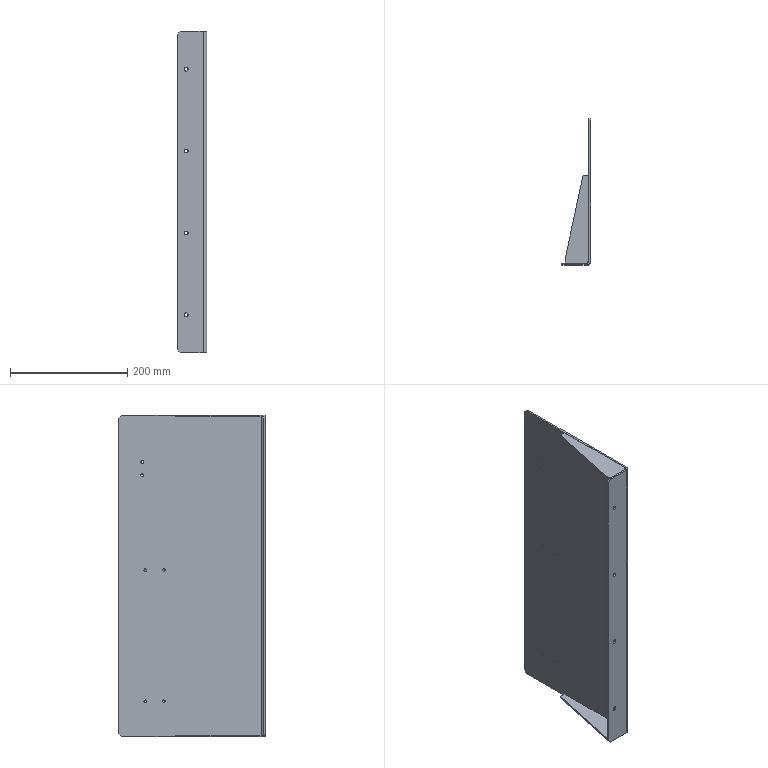Part | SolidWorks | features BaseBody 3 | 3 solids | 50 faces | box 50 x 250 x 550 mm | volume 509344 mm3 | plane 28 | cylinder 22 | commonest cylinder face diameters 4.2 x8 6.6 x8 5 x4 6 x1 12 x1
STEP:
#1=CARTESIAN_POINT('',(-3.,8.,272.));
#2=VERTEX_POINT('',#1);
#3=CARTESIAN_POINT('',(-8.,3.,272.));
#4=VERTEX_POINT('',#3);
#5=CARTESIAN_POINT('',(-5.5,5.5,272.));
#6=DIRECTION('',(-0.7071,-0.7071,0.));
#7=VECTOR('',#6,1000.);
#8=LINE('',#5,#7);
#9=EDGE_CURVE('',#2,#4,#8,.T.);
#10=ORIENTED_EDGE('',*,*,#9,.F.);
#11=CARTESIAN_POINT('',(-3.,8.,275.));
#12=VERTEX_POINT('',#11);
#13=CARTESIAN_POINT('',(-3.,8.,272.));
#14=DIRECTION('',(0.,0.,-1.));
#15=VECTOR('',#14,1000.);
#16=LINE('',#13,#15);
#17=EDGE_CURVE('',#12,#2,#16,.T.);
#18=ORIENTED_EDGE('',*,*,#17,.F.);
#19=CARTESIAN_POINT('',(-8.,3.,275.));
#20=VERTEX_POINT('',#19);
#21=CARTESIAN_POINT('',(-8.,3.,275.));
#22=DIRECTION('',(0.7071,0.7071,0.));
#23=VECTOR('',#22,1000.);
#24=LINE('',#21,#23);
#25=EDGE_CURVE('',#20,#12,#24,.T.);
#26=ORIENTED_EDGE('',*,*,#25,.F.);
#27=CARTESIAN_POINT('',(-8.,3.,272.));
#28=DIRECTION('',(0.,0.,1.));
#29=VECTOR('',#28,1000.);
#30=LINE('',#27,#29);
#31=EDGE_CURVE('',#4,#20,#30,.T.);
#32=ORIENTED_EDGE('',*,*,#31,.F.);
#33=EDGE_LOOP('',(#10,#18,#26,#32));
#34=FACE_OUTER_BOUND('',#33,.T.);
#35=CARTESIAN_POINT('',(-8.,3.,272.));
#36=DIRECTION('',(-0.7071,0.7071,0.));
#37=DIRECTION('',(0.,0.,1.));
#38=AXIS2_PLACEMENT_3D('',#35,#36,#37);
#39=PLANE('',#38);
#40=ADVANCED_FACE('',(#34),#39,.F.);
#41=CARTESIAN_POINT('',(-43.,3.,275.));
#42=VERTEX_POINT('',#41);
#43=CARTESIAN_POINT('',(-3.,3.,275.));
#44=DIRECTION('',(-1.,0.,0.));
#45=VECTOR('',#44,1000.);
#46=LINE('',#43,#45);
#47=EDGE_CURVE('',#20,#42,#46,.T.);
#48=ORIENTED_EDGE('',*,*,#47,.F.);
#49=ORIENTED_EDGE('',*,*,#25,.T.);
#50=CARTESIAN_POINT('',(-3.,153.,275.));
#51=VERTEX_POINT('',#50);
#52=CARTESIAN_POINT('',(-3.,3.,275.));
#53=DIRECTION('',(0.,-1.,0.));
#54=VECTOR('',#53,1000.);
#55=LINE('',#52,#54);
#56=EDGE_CURVE('',#51,#12,#55,.T.);
#57=ORIENTED_EDGE('',*,*,#56,.F.);
#58=CARTESIAN_POINT('',(-13.,153.,275.));
#59=VERTEX_POINT('',#58);
#60=CARTESIAN_POINT('',(-3.,153.,275.));
#61=DIRECTION('',(1.,0.,0.));
#62=VECTOR('',#61,1000.);
#63=LINE('',#60,#62);
#64=EDGE_CURVE('',#59,#51,#63,.T.);
#65=ORIENTED_EDGE('',*,*,#64,.F.);
#66=CARTESIAN_POINT('',(-43.,13.,275.));
#67=VERTEX_POINT('',#66);
#68=CARTESIAN_POINT('',(-13.,153.,275.));
#69=DIRECTION('',(0.2095,0.9778,0.));
#70=VECTOR('',#69,1000.);
#71=LINE('',#68,#70);
#72=EDGE_CURVE('',#67,#59,#71,.T.);
#73=ORIENTED_EDGE('',*,*,#72,.F.);
#74=CARTESIAN_POINT('',(-43.,3.,275.));
#75=DIRECTION('',(0.,1.,0.));
#76=VECTOR('',#75,1000.);
#77=LINE('',#74,#76);
#78=EDGE_CURVE('',#42,#67,#77,.T.);
#79=ORIENTED_EDGE('',*,*,#78,.F.);
#80=EDGE_LOOP('',(#48,#49,#57,#65,#73,#79));
#81=FACE_OUTER_BOUND('',#80,.T.);
#82=CARTESIAN_POINT('',(0.,0.,275.));
#83=DIRECTION('',(0.,0.,-1.));
#84=DIRECTION('',(-1.,0.,0.));
#85=AXIS2_PLACEMENT_3D('',#82,#83,#84);
#86=PLANE('',#85);
#87=ADVANCED_FACE('',(#81),#86,.F.);
#88=CARTESIAN_POINT('',(-3.,153.,272.));
#89=VERTEX_POINT('',#88);
#90=CARTESIAN_POINT('',(-3.,3.,272.));
#91=DIRECTION('',(0.,-1.,0.));
#92=VECTOR('',#91,1000.);
#93=LINE('',#90,#92);
#94=EDGE_CURVE('',#89,#2,#93,.T.);
#95=ORIENTED_EDGE('',*,*,#94,.T.);
#96=ORIENTED_EDGE('',*,*,#9,.T.);
#97=CARTESIAN_POINT('',(-43.,3.,272.));
#98=VERTEX_POINT('',#97);
#99=CARTESIAN_POINT('',(-3.,3.,272.));
#100=DIRECTION('',(-1.,0.,0.));
#101=VECTOR('',#100,1000.);
#102=LINE('',#99,#101);
#103=EDGE_CURVE('',#4,#98,#102,.T.);
#104=ORIENTED_EDGE('',*,*,#103,.T.);
#105=CARTESIAN_POINT('',(-43.,13.,272.));
#106=VERTEX_POINT('',#105);
#107=CARTESIAN_POINT('',(-43.,3.,272.));
#108=DIRECTION('',(0.,1.,0.));
#109=VECTOR('',#108,1000.);
#110=LINE('',#107,#109);
#111=EDGE_CURVE('',#98,#106,#110,.T.);
#112=ORIENTED_EDGE('',*,*,#111,.T.);
#113=CARTESIAN_POINT('',(-13.,153.,272.));
#114=VERTEX_POINT('',#113);
#115=CARTESIAN_POINT('',(-13.,153.,272.));
#116=DIRECTION('',(0.2095,0.9778,0.));
#117=VECTOR('',#116,1000.);
#118=LINE('',#115,#117);
#119=EDGE_CURVE('',#106,#114,#118,.T.);
#120=ORIENTED_EDGE('',*,*,#119,.T.);
#121=CARTESIAN_POINT('',(-3.,153.,272.));
#122=DIRECTION('',(1.,0.,0.));
#123=VECTOR('',#122,1000.);
#124=LINE('',#121,#123);
#125=EDGE_CURVE('',#114,#89,#124,.T.);
#126=ORIENTED_EDGE('',*,*,#125,.T.);
#127=EDGE_LOOP('',(#95,#96,#104,#112,#120,#126));
#128=FACE_OUTER_BOUND('',#127,.T.);
#129=CARTESIAN_POINT('',(0.,0.,272.));
#130=DIRECTION('',(0.,0.,-1.));
#131=DIRECTION('',(-1.,0.,0.));
#132=AXIS2_PLACEMENT_3D('',#129,#130,#131);
#133=PLANE('',#132);
#134=ADVANCED_FACE('',(#128),#133,.T.);
#135=ORIENTED_EDGE('',*,*,#72,.T.);
#136=CARTESIAN_POINT('',(-13.,153.,272.));
#137=DIRECTION('',(0.,0.,1.));
#138=VECTOR('',#137,1000.);
#139=LINE('',#136,#138);
#140=EDGE_CURVE('',#114,#59,#139,.T.);
#141=ORIENTED_EDGE('',*,*,#140,.F.);
#142=ORIENTED_EDGE('',*,*,#119,.F.);
#143=CARTESIAN_POINT('',(-43.,13.,272.));
#144=DIRECTION('',(0.,0.,1.));
#145=VECTOR('',#144,1000.);
#146=LINE('',#143,#145);
#147=EDGE_CURVE('',#106,#67,#146,.T.);
#148=ORIENTED_EDGE('',*,*,#147,.T.);
#149=EDGE_LOOP('',(#135,#141,#142,#148));
#150=FACE_OUTER_BOUND('',#149,.T.);
#151=CARTESIAN_POINT('',(-13.,153.,272.));
#152=DIRECTION('',(0.9778,-0.2095,0.));
#153=DIRECTION('',(0.,0.,-1.));
#154=AXIS2_PLACEMENT_3D('',#151,#152,#153);
#155=PLANE('',#154);
#156=ADVANCED_FACE('',(#150),#155,.F.);
#157=ORIENTED_EDGE('',*,*,#78,.T.);
#158=ORIENTED_EDGE('',*,*,#147,.F.);
#159=ORIENTED_EDGE('',*,*,#111,.F.);
#160=CARTESIAN_POINT('',(-43.,3.,272.));
#161=DIRECTION('',(0.,0.,1.));
#162=VECTOR('',#161,1000.);
#163=LINE('',#160,#162);
#164=EDGE_CURVE('',#98,#42,#163,.T.);
#165=ORIENTED_EDGE('',*,*,#164,.T.);
#166=EDGE_LOOP('',(#157,#158,#159,#165));
#167=FACE_OUTER_BOUND('',#166,.T.);
#168=CARTESIAN_POINT('',(-43.,3.,272.));
#169=DIRECTION('',(1.,0.,0.));
#170=DIRECTION('',(0.,1.,0.));
#171=AXIS2_PLACEMENT_3D('',#168,#169,#170);
#172=PLANE('',#171);
#173=ADVANCED_FACE('',(#167),#172,.F.);
#174=ORIENTED_EDGE('',*,*,#103,.F.);
#175=ORIENTED_EDGE('',*,*,#31,.T.);
#176=ORIENTED_EDGE('',*,*,#47,.T.);
#177=ORIENTED_EDGE('',*,*,#164,.F.);
#178=EDGE_LOOP('',(#174,#175,#176,#177));
#179=FACE_OUTER_BOUND('',#178,.T.);
#180=CARTESIAN_POINT('',(-3.,3.,272.));
#181=DIRECTION('',(0.,1.,0.));
#182=DIRECTION('',(1.,0.,0.));
#183=AXIS2_PLACEMENT_3D('',#180,#181,#182);
#184=PLANE('',#183);
#185=ADVANCED_FACE('',(#179),#184,.F.);
#186=ORIENTED_EDGE('',*,*,#56,.T.);
#187=ORIENTED_EDGE('',*,*,#17,.T.);
#188=ORIENTED_EDGE('',*,*,#94,.F.);
#189=CARTESIAN_POINT('',(-3.,153.,272.));
#190=DIRECTION('',(0.,0.,1.));
#191=VECTOR('',#190,1000.);
#192=LINE('',#189,#191);
#193=EDGE_CURVE('',#89,#51,#192,.T.);
#194=ORIENTED_EDGE('',*,*,#193,.T.);
#195=EDGE_LOOP('',(#186,#187,#188,#194));
#196=FACE_OUTER_BOUND('',#195,.T.);
#197=CARTESIAN_POINT('',(-3.,3.,272.));
#198=DIRECTION('',(-1.,0.,0.));
#199=DIRECTION('',(0.,1.,0.));
#200=AXIS2_PLACEMENT_3D('',#197,#198,#199);
#201=PLANE('',#200);
#202=ADVANCED_FACE('',(#196),#201,.F.);
#203=ORIENTED_EDGE('',*,*,#64,.T.);
#204=ORIENTED_EDGE('',*,*,#193,.F.);
#205=ORIENTED_EDGE('',*,*,#125,.F.);
#206=ORIENTED_EDGE('',*,*,#140,.T.);
#207=EDGE_LOOP('',(#203,#204,#205,#206));
#208=FACE_OUTER_BOUND('',#207,.T.);
#209=CARTESIAN_POINT('',(-3.,153.,272.));
#210=DIRECTION('',(0.,-1.,0.));
#211=DIRECTION('',(-1.,0.,0.));
#212=AXIS2_PLACEMENT_3D('',#209,#210,#211);
#213=PLANE('',#212);
#214=ADVANCED_FACE('',(#208),#213,.F.);
#215=CLOSED_SHELL('',(#40,#87,#134,#156,#173,#185,#202,#214));
#216=MANIFOLD_SOLID_BREP('',#215);
#217=CARTESIAN_POINT('',(-8.,3.,-272.));
#218=VERTEX_POINT('',#217);
#219=CARTESIAN_POINT('',(-3.,8.,-272.));
#220=VERTEX_POINT('',#219);
#221=CARTESIAN_POINT('',(-3.,8.,-272.));
#222=DIRECTION('',(0.7071,0.7071,0.));
#223=VECTOR('',#222,1000.);
#224=LINE('',#221,#223);
#225=EDGE_CURVE('',#218,#220,#224,.T.);
#226=ORIENTED_EDGE('',*,*,#225,.F.);
#227=CARTESIAN_POINT('',(-8.,3.,-275.));
#228=VERTEX_POINT('',#227);
#229=CARTESIAN_POINT('',(-8.,3.,-272.));
#230=DIRECTION('',(0.,0.,1.));
#231=VECTOR('',#230,1000.);
#232=LINE('',#229,#231);
#233=EDGE_CURVE('',#228,#218,#232,.T.);
#234=ORIENTED_EDGE('',*,*,#233,.F.);
#235=CARTESIAN_POINT('',(-3.,8.,-275.));
#236=VERTEX_POINT('',#235);
#237=CARTESIAN_POINT('',(-5.5,5.5,-275.));
#238=DIRECTION('',(-0.7071,-0.7071,0.));
#239=VECTOR('',#238,1000.);
#240=LINE('',#237,#239);
#241=EDGE_CURVE('',#236,#228,#240,.T.);
#242=ORIENTED_EDGE('',*,*,#241,.F.);
#243=CARTESIAN_POINT('',(-3.,8.,-272.));
#244=DIRECTION('',(0.,0.,-1.));
#245=VECTOR('',#244,1000.);
#246=LINE('',#243,#245);
#247=EDGE_CURVE('',#220,#236,#246,.T.);
#248=ORIENTED_EDGE('',*,*,#247,.F.);
#249=EDGE_LOOP('',(#226,#234,#242,#248));
#250=FACE_OUTER_BOUND('',#249,.T.);
#251=CARTESIAN_POINT('',(-3.,8.,-272.));
#252=DIRECTION('',(-0.7071,0.7071,0.));
#253=DIRECTION('',(0.,0.,1.));
#254=AXIS2_PLACEMENT_3D('',#251,#252,#253);
#255=PLANE('',#254);
#256=ADVANCED_FACE('',(#250),#255,.F.);
#257=CARTESIAN_POINT('',(-3.,153.,-275.));
#258=VERTEX_POINT('',#257);
#259=CARTESIAN_POINT('',(-3.,3.,-275.));
#260=DIRECTION('',(0.,1.,0.));
#261=VECTOR('',#260,1000.);
#262=LINE('',#259,#261);
#263=EDGE_CURVE('',#236,#258,#262,.T.);
#264=ORIENTED_EDGE('',*,*,#263,.F.);
#265=ORIENTED_EDGE('',*,*,#241,.T.);
#266=CARTESIAN_POINT('',(-43.,3.,-275.));
#267=VERTEX_POINT('',#266);
#268=CARTESIAN_POINT('',(-3.,3.,-275.));
#269=DIRECTION('',(1.,0.,0.));
#270=VECTOR('',#269,1000.);
#271=LINE('',#268,#270);
#272=EDGE_CURVE('',#267,#228,#271,.T.);
#273=ORIENTED_EDGE('',*,*,#272,.F.);
#274=CARTESIAN_POINT('',(-43.,13.,-275.));
#275=VERTEX_POINT('',#274);
#276=CARTESIAN_POINT('',(-43.,3.,-275.));
#277=DIRECTION('',(0.,-1.,0.));
#278=VECTOR('',#277,1000.);
#279=LINE('',#276,#278);
#280=EDGE_CURVE('',#275,#267,#279,.T.);
#281=ORIENTED_EDGE('',*,*,#280,.F.);
#282=CARTESIAN_POINT('',(-13.,153.,-275.));
#283=VERTEX_POINT('',#282);
#284=CARTESIAN_POINT('',(-13.,153.,-275.));
#285=DIRECTION('',(-0.2095,-0.9778,0.));
#286=VECTOR('',#285,1000.);
#287=LINE('',#284,#286);
#288=EDGE_CURVE('',#283,#275,#287,.T.);
#289=ORIENTED_EDGE('',*,*,#288,.F.);
#290=CARTESIAN_POINT('',(-3.,153.,-275.));
#291=DIRECTION('',(-1.,0.,0.));
#292=VECTOR('',#291,1000.);
#293=LINE('',#290,#292);
#294=EDGE_CURVE('',#258,#283,#293,.T.);
#295=ORIENTED_EDGE('',*,*,#294,.F.);
#296=EDGE_LOOP('',(#264,#265,#273,#281,#289,#295));
#297=FACE_OUTER_BOUND('',#296,.T.);
#298=CARTESIAN_POINT('',(0.,0.,-275.));
#299=DIRECTION('',(0.,0.,-1.));
#300=DIRECTION('',(-1.,0.,0.));
#301=AXIS2_PLACEMENT_3D('',#298,#299,#300);
#302=PLANE('',#301);
#303=ADVANCED_FACE('',(#297),#302,.T.);
#304=CARTESIAN_POINT('',(-43.,3.,-272.));
#305=VERTEX_POINT('',#304);
#306=CARTESIAN_POINT('',(-3.,3.,-272.));
#307=DIRECTION('',(1.,0.,0.));
#308=VECTOR('',#307,1000.);
#309=LINE('',#306,#308);
#310=EDGE_CURVE('',#305,#218,#309,.T.);
#311=ORIENTED_EDGE('',*,*,#310,.T.);
#312=ORIENTED_EDGE('',*,*,#225,.T.);
#313=CARTESIAN_POINT('',(-3.,153.,-272.));
#314=VERTEX_POINT('',#313);
#315=CARTESIAN_POINT('',(-3.,3.,-272.));
#316=DIRECTION('',(0.,1.,0.));
#317=VECTOR('',#316,1000.);
#318=LINE('',#315,#317);
#319=EDGE_CURVE('',#220,#314,#318,.T.);
#320=ORIENTED_EDGE('',*,*,#319,.T.);
#321=CARTESIAN_POINT('',(-13.,153.,-272.));
#322=VERTEX_POINT('',#321);
#323=CARTESIAN_POINT('',(-3.,153.,-272.));
#324=DIRECTION('',(-1.,0.,0.));
#325=VECTOR('',#324,1000.);
#326=LINE('',#323,#325);
#327=EDGE_CURVE('',#314,#322,#326,.T.);
#328=ORIENTED_EDGE('',*,*,#327,.T.);
#329=CARTESIAN_POINT('',(-43.,13.,-272.));
#330=VERTEX_POINT('',#329);
#331=CARTESIAN_POINT('',(-13.,153.,-272.));
#332=DIRECTION('',(-0.2095,-0.9778,0.));
#333=VECTOR('',#332,1000.);
#334=LINE('',#331,#333);
#335=EDGE_CURVE('',#322,#330,#334,.T.);
#336=ORIENTED_EDGE('',*,*,#335,.T.);
#337=CARTESIAN_POINT('',(-43.,3.,-272.));
#338=DIRECTION('',(0.,-1.,0.));
#339=VECTOR('',#338,1000.);
#340=LINE('',#337,#339);
#341=EDGE_CURVE('',#330,#305,#340,.T.);
#342=ORIENTED_EDGE('',*,*,#341,.T.);
#343=EDGE_LOOP('',(#311,#312,#320,#328,#336,#342));
#344=FACE_OUTER_BOUND('',#343,.T.);
#345=CARTESIAN_POINT('',(0.,0.,-272.));
#346=DIRECTION('',(0.,0.,-1.));
#347=DIRECTION('',(-1.,0.,0.));
#348=AXIS2_PLACEMENT_3D('',#345,#346,#347);
#349=PLANE('',#348);
#350=ADVANCED_FACE('',(#344),#349,.F.);
#351=ORIENTED_EDGE('',*,*,#319,.F.);
#352=ORIENTED_EDGE('',*,*,#247,.T.);
#353=ORIENTED_EDGE('',*,*,#263,.T.);
#354=CARTESIAN_POINT('',(-3.,153.,-272.));
#355=DIRECTION('',(0.,0.,-1.));
#356=VECTOR('',#355,1000.);
#357=LINE('',#354,#356);
#358=EDGE_CURVE('',#314,#258,#357,.T.);
#359=ORIENTED_EDGE('',*,*,#358,.F.);
#360=EDGE_LOOP('',(#351,#352,#353,#359));
#361=FACE_OUTER_BOUND('',#360,.T.);
#362=CARTESIAN_POINT('',(-3.,3.,-272.));
#363=DIRECTION('',(-1.,0.,0.));
#364=DIRECTION('',(0.,1.,0.));
#365=AXIS2_PLACEMENT_3D('',#362,#363,#364);
#366=PLANE('',#365);
#367=ADVANCED_FACE('',(#361),#366,.F.);
#368=ORIENTED_EDGE('',*,*,#272,.T.);
#369=ORIENTED_EDGE('',*,*,#233,.T.);
#370=ORIENTED_EDGE('',*,*,#310,.F.);
#371=CARTESIAN_POINT('',(-43.,3.,-272.));
#372=DIRECTION('',(0.,0.,-1.));
#373=VECTOR('',#372,1000.);
#374=LINE('',#371,#373);
#375=EDGE_CURVE('',#305,#267,#374,.T.);
#376=ORIENTED_EDGE('',*,*,#375,.T.);
#377=EDGE_LOOP('',(#368,#369,#370,#376));
#378=FACE_OUTER_BOUND('',#377,.T.);
#379=CARTESIAN_POINT('',(-3.,3.,-272.));
#380=DIRECTION('',(0.,1.,0.));
#381=DIRECTION('',(0.,0.,-1.));
#382=AXIS2_PLACEMENT_3D('',#379,#380,#381);
#383=PLANE('',#382);
#384=ADVANCED_FACE('',(#378),#383,.F.);
#385=ORIENTED_EDGE('',*,*,#280,.T.);
#386=ORIENTED_EDGE('',*,*,#375,.F.);
#387=ORIENTED_EDGE('',*,*,#341,.F.);
#388=CARTESIAN_POINT('',(-43.,13.,-272.));
#389=DIRECTION('',(0.,0.,-1.));
#390=VECTOR('',#389,1000.);
#391=LINE('',#388,#390);
#392=EDGE_CURVE('',#330,#275,#391,.T.);
#393=ORIENTED_EDGE('',*,*,#392,.T.);
#394=EDGE_LOOP('',(#385,#386,#387,#393));
#395=FACE_OUTER_BOUND('',#394,.T.);
#396=CARTESIAN_POINT('',(-43.,3.,-272.));
#397=DIRECTION('',(1.,0.,0.));
#398=DIRECTION('',(0.,-1.,0.));
#399=AXIS2_PLACEMENT_3D('',#396,#397,#398);
#400=PLANE('',#399);
#401=ADVANCED_FACE('',(#395),#400,.F.);
#402=ORIENTED_EDGE('',*,*,#288,.T.);
#403=ORIENTED_EDGE('',*,*,#392,.F.);
#404=ORIENTED_EDGE('',*,*,#335,.F.);
#405=CARTESIAN_POINT('',(-13.,153.,-272.));
#406=DIRECTION('',(0.,0.,-1.));
#407=VECTOR('',#406,1000.);
#408=LINE('',#405,#407);
#409=EDGE_CURVE('',#322,#283,#408,.T.);
#410=ORIENTED_EDGE('',*,*,#409,.T.);
#411=EDGE_LOOP('',(#402,#403,#404,#410));
#412=FACE_OUTER_BOUND('',#411,.T.);
#413=CARTESIAN_POINT('',(-13.,153.,-272.));
#414=DIRECTION('',(0.9778,-0.2095,0.));
#415=DIRECTION('',(0.,0.,-1.));
#416=AXIS2_PLACEMENT_3D('',#413,#414,#415);
#417=PLANE('',#416);
#418=ADVANCED_FACE('',(#412),#417,.F.);
#419=ORIENTED_EDGE('',*,*,#294,.T.);
#420=ORIENTED_EDGE('',*,*,#409,.F.);
#421=ORIENTED_EDGE('',*,*,#327,.F.);
#422=ORIENTED_EDGE('',*,*,#358,.T.);
#423=EDGE_LOOP('',(#419,#420,#421,#422));
#424=FACE_OUTER_BOUND('',#423,.T.);
#425=CARTESIAN_POINT('',(-3.,153.,-272.));
#426=DIRECTION('',(0.,-1.,0.));
#427=DIRECTION('',(0.,0.,-1.));
#428=AXIS2_PLACEMENT_3D('',#425,#426,#427);
#429=PLANE('',#428);
#430=ADVANCED_FACE('',(#424),#429,.F.);
#431=CLOSED_SHELL('',(#256,#303,#350,#367,#384,#401,#418,#430));
#432=MANIFOLD_SOLID_BREP('',#431);
#433=CARTESIAN_POINT('',(-3.,210.,197.5));
#434=VERTEX_POINT('',#433);
#435=CARTESIAN_POINT('',(-3.,210.,192.5));
#436=VERTEX_POINT('',#435);
#437=CARTESIAN_POINT('',(-3.,210.,195.));
#438=DIRECTION('',(1.,0.,0.));
#439=DIRECTION('',(0.,1.,0.));
#440=AXIS2_PLACEMENT_3D('',#437,#438,#439);
#441=CIRCLE('',#440,2.5);
#442=EDGE_CURVE('',#434,#436,#441,.T.);
#443=ORIENTED_EDGE('',*,*,#442,.F.);
#444=CARTESIAN_POINT('',(0.,210.,197.5));
#445=VERTEX_POINT('',#444);
#446=CARTESIAN_POINT('',(0.,210.,197.5));
#447=DIRECTION('',(1.,0.,0.));
#448=VECTOR('',#447,1000.);
#449=LINE('',#446,#448);
#450=EDGE_CURVE('',#434,#445,#449,.T.);
#451=ORIENTED_EDGE('',*,*,#450,.T.);
#452=CARTESIAN_POINT('',(0.,210.,192.5));
#453=VERTEX_POINT('',#452);
#454=CARTESIAN_POINT('',(0.,210.,195.));
#455=DIRECTION('',(1.,0.,0.));
#456=DIRECTION('',(0.,0.,-1.));
#457=AXIS2_PLACEMENT_3D('',#454,#455,#456);
#458=CIRCLE('',#457,2.5);
#459=EDGE_CURVE('',#445,#453,#458,.T.);
#460=ORIENTED_EDGE('',*,*,#459,.T.);
#461=CARTESIAN_POINT('',(0.,210.,192.5));
#462=DIRECTION('',(1.,0.,0.));
#463=VECTOR('',#462,1000.);
#464=LINE('',#461,#463);
#465=EDGE_CURVE('',#436,#453,#464,.T.);
#466=ORIENTED_EDGE('',*,*,#465,.F.);
#467=EDGE_LOOP('',(#443,#451,#460,#466));
#468=FACE_OUTER_BOUND('',#467,.T.);
#469=CARTESIAN_POINT('',(0.,210.,195.));
#470=DIRECTION('',(1.,0.,0.));
#471=DIRECTION('',(0.,0.,-1.));
#472=AXIS2_PLACEMENT_3D('',#469,#470,#471);
#473=CYLINDRICAL_SURFACE('',#472,2.5);
#474=ADVANCED_FACE('',(#468),#473,.F.);
#475=CARTESIAN_POINT('',(-3.,210.,174.5));
#476=VERTEX_POINT('',#475);
#477=CARTESIAN_POINT('',(-3.,210.,169.5));
#478=VERTEX_POINT('',#477);
#479=CARTESIAN_POINT('',(-3.,210.,172.));
#480=DIRECTION('',(1.,0.,0.));
#481=DIRECTION('',(0.,1.,0.));
#482=AXIS2_PLACEMENT_3D('',#479,#480,#481);
#483=CIRCLE('',#482,2.5);
#484=EDGE_CURVE('',#476,#478,#483,.T.);
#485=ORIENTED_EDGE('',*,*,#484,.F.);
#486=CARTESIAN_POINT('',(0.,210.,174.5));
#487=VERTEX_POINT('',#486);
#488=CARTESIAN_POINT('',(0.,210.,174.5));
#489=DIRECTION('',(1.,0.,0.));
#490=VECTOR('',#489,1000.);
#491=LINE('',#488,#490);
#492=EDGE_CURVE('',#476,#487,#491,.T.);
#493=ORIENTED_EDGE('',*,*,#492,.T.);
#494=CARTESIAN_POINT('',(0.,210.,169.5));
#495=VERTEX_POINT('',#494);
#496=CARTESIAN_POINT('',(0.,210.,172.));
#497=DIRECTION('',(1.,0.,0.));
#498=DIRECTION('',(0.,0.,-1.));
#499=AXIS2_PLACEMENT_3D('',#496,#497,#498);
#500=CIRCLE('',#499,2.5);
#501=EDGE_CURVE('',#487,#495,#500,.T.);
#502=ORIENTED_EDGE('',*,*,#501,.T.);
#503=CARTESIAN_POINT('',(0.,210.,169.5));
#504=DIRECTION('',(1.,0.,0.));
#505=VECTOR('',#504,1000.);
#506=LINE('',#503,#505);
#507=EDGE_CURVE('',#478,#495,#506,.T.);
#508=ORIENTED_EDGE('',*,*,#507,.F.);
#509=EDGE_LOOP('',(#485,#493,#502,#508));
#510=FACE_OUTER_BOUND('',#509,.T.);
#511=CARTESIAN_POINT('',(0.,210.,172.));
#512=DIRECTION('',(1.,0.,0.));
#513=DIRECTION('',(0.,0.,-1.));
#514=AXIS2_PLACEMENT_3D('',#511,#512,#513);
#515=CYLINDRICAL_SURFACE('',#514,2.5);
#516=ADVANCED_FACE('',(#510),#515,.F.);
#517=CARTESIAN_POINT('',(-35.,0.,213.3));
#518=VERTEX_POINT('',#517);
#519=CARTESIAN_POINT('',(-35.,0.,206.7));
#520=VERTEX_POINT('',#519);
#521=CARTESIAN_POINT('',(-35.,0.,210.));
#522=DIRECTION('',(0.,-1.,0.));
#523=DIRECTION('',(0.,0.,-1.));
#524=AXIS2_PLACEMENT_3D('',#521,#522,#523);
#525=CIRCLE('',#524,3.3);
#526=EDGE_CURVE('',#518,#520,#525,.T.);
#527=ORIENTED_EDGE('',*,*,#526,.T.);
#528=CARTESIAN_POINT('',(-35.,3.,206.7));
#529=VERTEX_POINT('',#528);
#530=CARTESIAN_POINT('',(-35.,3.,206.7));
#531=DIRECTION('',(0.,1.,0.));
#532=VECTOR('',#531,1000.);
#533=LINE('',#530,#532);
#534=EDGE_CURVE('',#520,#529,#533,.T.);
#535=ORIENTED_EDGE('',*,*,#534,.T.);
#536=CARTESIAN_POINT('',(-35.,3.,213.3));
#537=VERTEX_POINT('',#536);
#538=CARTESIAN_POINT('',(-35.,3.,210.));
#539=DIRECTION('',(0.,1.,0.));
#540=DIRECTION('',(0.,0.,1.));
#541=AXIS2_PLACEMENT_3D('',#538,#539,#540);
#542=CIRCLE('',#541,3.3);
#543=EDGE_CURVE('',#529,#537,#542,.T.);
#544=ORIENTED_EDGE('',*,*,#543,.T.);
#545=CARTESIAN_POINT('',(-35.,3.,213.3));
#546=DIRECTION('',(0.,1.,0.));
#547=VECTOR('',#546,1000.);
#548=LINE('',#545,#547);
#549=EDGE_CURVE('',#518,#537,#548,.T.);
#550=ORIENTED_EDGE('',*,*,#549,.F.);
#551=EDGE_LOOP('',(#527,#535,#544,#550));
#552=FACE_OUTER_BOUND('',#551,.T.);
#553=CARTESIAN_POINT('',(-35.,3.,210.));
#554=DIRECTION('',(0.,1.,0.));
#555=DIRECTION('',(0.,0.,1.));
#556=AXIS2_PLACEMENT_3D('',#553,#554,#555);
#557=CYLINDRICAL_SURFACE('',#556,3.3);
#558=ADVANCED_FACE('',(#552),#557,.F.);
#559=CARTESIAN_POINT('',(-35.,0.,-206.7));
#560=VERTEX_POINT('',#559);
#561=CARTESIAN_POINT('',(-35.,0.,-213.3));
#562=VERTEX_POINT('',#561);
#563=CARTESIAN_POINT('',(-35.,0.,-210.));
#564=DIRECTION('',(0.,-1.,0.));
#565=DIRECTION('',(0.,0.,-1.));
#566=AXIS2_PLACEMENT_3D('',#563,#564,#565);
#567=CIRCLE('',#566,3.3);
#568=EDGE_CURVE('',#560,#562,#567,.T.);
#569=ORIENTED_EDGE('',*,*,#568,.T.);
#570=CARTESIAN_POINT('',(-35.,3.,-213.3));
#571=VERTEX_POINT('',#570);
#572=CARTESIAN_POINT('',(-35.,3.,-213.3));
#573=DIRECTION('',(0.,1.,0.));
#574=VECTOR('',#573,1000.);
#575=LINE('',#572,#574);
#576=EDGE_CURVE('',#562,#571,#575,.T.);
#577=ORIENTED_EDGE('',*,*,#576,.T.);
#578=CARTESIAN_POINT('',(-35.,3.,-206.7));
#579=VERTEX_POINT('',#578);
#580=CARTESIAN_POINT('',(-35.,3.,-210.));
#581=DIRECTION('',(0.,1.,0.));
#582=DIRECTION('',(0.,0.,1.));
#583=AXIS2_PLACEMENT_3D('',#580,#581,#582);
#584=CIRCLE('',#583,3.3);
#585=EDGE_CURVE('',#571,#579,#584,.T.);
#586=ORIENTED_EDGE('',*,*,#585,.T.);
#587=CARTESIAN_POINT('',(-35.,3.,-206.7));
#588=DIRECTION('',(0.,1.,0.));
#589=VECTOR('',#588,1000.);
#590=LINE('',#587,#589);
#591=EDGE_CURVE('',#560,#579,#590,.T.);
#592=ORIENTED_EDGE('',*,*,#591,.F.);
#593=EDGE_LOOP('',(#569,#577,#586,#592));
#594=FACE_OUTER_BOUND('',#593,.T.);
#595=CARTESIAN_POINT('',(-35.,3.,-210.));
#596=DIRECTION('',(0.,1.,0.));
#597=DIRECTION('',(0.,0.,1.));
#598=AXIS2_PLACEMENT_3D('',#595,#596,#597);
#599=CYLINDRICAL_SURFACE('',#598,3.3);
#600=ADVANCED_FACE('',(#594),#599,.F.);
#601=CARTESIAN_POINT('',(-35.,0.,73.3));
#602=VERTEX_POINT('',#601);
#603=CARTESIAN_POINT('',(-35.,0.,66.7));
#604=VERTEX_POINT('',#603);
#605=CARTESIAN_POINT('',(-35.,0.,70.));
#606=DIRECTION('',(0.,-1.,0.));
#607=DIRECTION('',(0.,0.,-1.));
#608=AXIS2_PLACEMENT_3D('',#605,#606,#607);
#609=CIRCLE('',#608,3.3);
#610=EDGE_CURVE('',#602,#604,#609,.T.);
#611=ORIENTED_EDGE('',*,*,#610,.T.);
#612=CARTESIAN_POINT('',(-35.,3.,66.7));
#613=VERTEX_POINT('',#612);
#614=CARTESIAN_POINT('',(-35.,3.,66.7));
#615=DIRECTION('',(0.,1.,0.));
#616=VECTOR('',#615,1000.);
#617=LINE('',#614,#616);
#618=EDGE_CURVE('',#604,#613,#617,.T.);
#619=ORIENTED_EDGE('',*,*,#618,.T.);
#620=CARTESIAN_POINT('',(-35.,3.,73.3));
#621=VERTEX_POINT('',#620);
#622=CARTESIAN_POINT('',(-35.,3.,70.));
#623=DIRECTION('',(0.,1.,0.));
#624=DIRECTION('',(0.,0.,1.));
#625=AXIS2_PLACEMENT_3D('',#622,#623,#624);
#626=CIRCLE('',#625,3.3);
#627=EDGE_CURVE('',#613,#621,#626,.T.);
#628=ORIENTED_EDGE('',*,*,#627,.T.);
#629=CARTESIAN_POINT('',(-35.,3.,73.3));
#630=DIRECTION('',(0.,1.,0.));
#631=VECTOR('',#630,1000.);
#632=LINE('',#629,#631);
#633=EDGE_CURVE('',#602,#621,#632,.T.);
#634=ORIENTED_EDGE('',*,*,#633,.F.);
#635=EDGE_LOOP('',(#611,#619,#628,#634));
#636=FACE_OUTER_BOUND('',#635,.T.);
#637=CARTESIAN_POINT('',(-35.,3.,70.));
#638=DIRECTION('',(0.,1.,0.));
#639=DIRECTION('',(0.,0.,1.));
#640=AXIS2_PLACEMENT_3D('',#637,#638,#639);
#641=CYLINDRICAL_SURFACE('',#640,3.3);
#642=ADVANCED_FACE('',(#636),#641,.F.);
#643=CARTESIAN_POINT('',(-35.,0.,-66.7));
#644=VERTEX_POINT('',#643);
#645=CARTESIAN_POINT('',(-35.,0.,-73.3));
#646=VERTEX_POINT('',#645);
#647=CARTESIAN_POINT('',(-35.,0.,-70.));
#648=DIRECTION('',(0.,-1.,0.));
#649=DIRECTION('',(0.,0.,-1.));
#650=AXIS2_PLACEMENT_3D('',#647,#648,#649);
#651=CIRCLE('',#650,3.3);
#652=EDGE_CURVE('',#644,#646,#651,.T.);
#653=ORIENTED_EDGE('',*,*,#652,.T.);
#654=CARTESIAN_POINT('',(-35.,3.,-73.3));
#655=VERTEX_POINT('',#654);
#656=CARTESIAN_POINT('',(-35.,3.,-73.3));
#657=DIRECTION('',(0.,1.,0.));
#658=VECTOR('',#657,1000.);
#659=LINE('',#656,#658);
#660=EDGE_CURVE('',#646,#655,#659,.T.);
#661=ORIENTED_EDGE('',*,*,#660,.T.);
#662=CARTESIAN_POINT('',(-35.,3.,-66.7));
#663=VERTEX_POINT('',#662);
#664=CARTESIAN_POINT('',(-35.,3.,-70.));
#665=DIRECTION('',(0.,1.,0.));
#666=DIRECTION('',(0.,0.,1.));
#667=AXIS2_PLACEMENT_3D('',#664,#665,#666);
#668=CIRCLE('',#667,3.3);
#669=EDGE_CURVE('',#655,#663,#668,.T.);
#670=ORIENTED_EDGE('',*,*,#669,.T.);
#671=CARTESIAN_POINT('',(-35.,3.,-66.7));
#672=DIRECTION('',(0.,1.,0.));
#673=VECTOR('',#672,1000.);
#674=LINE('',#671,#673);
#675=EDGE_CURVE('',#644,#663,#674,.T.);
#676=ORIENTED_EDGE('',*,*,#675,.F.);
#677=EDGE_LOOP('',(#653,#661,#670,#676));
#678=FACE_OUTER_BOUND('',#677,.T.);
#679=CARTESIAN_POINT('',(-35.,3.,-70.));
#680=DIRECTION('',(0.,1.,0.));
#681=DIRECTION('',(0.,0.,1.));
#682=AXIS2_PLACEMENT_3D('',#679,#680,#681);
#683=CYLINDRICAL_SURFACE('',#682,3.3);
#684=ADVANCED_FACE('',(#678),#683,.F.);
#685=CARTESIAN_POINT('',(-3.,205.,12.1));
#686=VERTEX_POINT('',#685);
#687=CARTESIAN_POINT('',(-3.,205.,7.9));
#688=VERTEX_POINT('',#687);
#689=CARTESIAN_POINT('',(-3.,205.,10.));
#690=DIRECTION('',(1.,0.,0.));
#691=DIRECTION('',(0.,1.,0.));
#692=AXIS2_PLACEMENT_3D('',#689,#690,#691);
#693=CIRCLE('',#692,2.1);
#694=EDGE_CURVE('',#686,#688,#693,.T.);
#695=ORIENTED_EDGE('',*,*,#694,.F.);
#696=CARTESIAN_POINT('',(0.,205.,12.1));
#697=VERTEX_POINT('',#696);
#698=CARTESIAN_POINT('',(0.,205.,12.1));
#699=DIRECTION('',(1.,0.,0.));
#700=VECTOR('',#699,1000.);
#701=LINE('',#698,#700);
#702=EDGE_CURVE('',#686,#697,#701,.T.);
#703=ORIENTED_EDGE('',*,*,#702,.T.);
#704=CARTESIAN_POINT('',(0.,205.,7.9));
#705=VERTEX_POINT('',#704);
#706=CARTESIAN_POINT('',(0.,205.,10.));
#707=DIRECTION('',(1.,0.,0.));
#708=DIRECTION('',(0.,0.,-1.));
#709=AXIS2_PLACEMENT_3D('',#706,#707,#708);
#710=CIRCLE('',#709,2.1);
#711=EDGE_CURVE('',#697,#705,#710,.T.);
#712=ORIENTED_EDGE('',*,*,#711,.T.);
#713=CARTESIAN_POINT('',(0.,205.,7.9));
#714=DIRECTION('',(1.,0.,0.));
#715=VECTOR('',#714,1000.);
#716=LINE('',#713,#715);
#717=EDGE_CURVE('',#688,#705,#716,.T.);
#718=ORIENTED_EDGE('',*,*,#717,.F.);
#719=EDGE_LOOP('',(#695,#703,#712,#718));
#720=FACE_OUTER_BOUND('',#719,.T.);
#721=CARTESIAN_POINT('',(0.,205.,10.));
#722=DIRECTION('',(1.,0.,0.));
#723=DIRECTION('',(0.,0.,-1.));
#724=AXIS2_PLACEMENT_3D('',#721,#722,#723);
#725=CYLINDRICAL_SURFACE('',#724,2.1);
#726=ADVANCED_FACE('',(#720),#725,.F.);
#727=CARTESIAN_POINT('',(-3.,173.,-211.9));
#728=VERTEX_POINT('',#727);
#729=CARTESIAN_POINT('',(-3.,173.,-216.1));
#730=VERTEX_POINT('',#729);
#731=CARTESIAN_POINT('',(-3.,173.,-214.));
#732=DIRECTION('',(1.,0.,0.));
#733=DIRECTION('',(0.,1.,0.));
#734=AXIS2_PLACEMENT_3D('',#731,#732,#733);
#735=CIRCLE('',#734,2.1);
#736=EDGE_CURVE('',#728,#730,#735,.T.);
#737=ORIENTED_EDGE('',*,*,#736,.F.);
#738=CARTESIAN_POINT('',(0.,173.,-211.9));
#739=VERTEX_POINT('',#738);
#740=CARTESIAN_POINT('',(0.,173.,-211.9));
#741=DIRECTION('',(1.,0.,0.));
#742=VECTOR('',#741,1000.);
#743=LINE('',#740,#742);
#744=EDGE_CURVE('',#728,#739,#743,.T.);
#745=ORIENTED_EDGE('',*,*,#744,.T.);
#746=CARTESIAN_POINT('',(0.,173.,-216.1));
#747=VERTEX_POINT('',#746);
#748=CARTESIAN_POINT('',(0.,173.,-214.));
#749=DIRECTION('',(1.,0.,0.));
#750=DIRECTION('',(0.,0.,-1.));
#751=AXIS2_PLACEMENT_3D('',#748,#749,#750);
#752=CIRCLE('',#751,2.1);
#753=EDGE_CURVE('',#739,#747,#752,.T.);
#754=ORIENTED_EDGE('',*,*,#753,.T.);
#755=CARTESIAN_POINT('',(0.,173.,-216.1));
#756=DIRECTION('',(1.,0.,0.));
#757=VECTOR('',#756,1000.);
#758=LINE('',#755,#757);
#759=EDGE_CURVE('',#730,#747,#758,.T.);
#760=ORIENTED_EDGE('',*,*,#759,.F.);
#761=EDGE_LOOP('',(#737,#745,#754,#760));
#762=FACE_OUTER_BOUND('',#761,.T.);
#763=CARTESIAN_POINT('',(0.,173.,-214.));
#764=DIRECTION('',(1.,0.,0.));
#765=DIRECTION('',(0.,0.,-1.));
#766=AXIS2_PLACEMENT_3D('',#763,#764,#765);
#767=CYLINDRICAL_SURFACE('',#766,2.1);
#768=ADVANCED_FACE('',(#762),#767,.F.);
#769=CARTESIAN_POINT('',(-3.,173.,12.1));
#770=VERTEX_POINT('',#769);
#771=CARTESIAN_POINT('',(-3.,173.,7.9));
#772=VERTEX_POINT('',#771);
#773=CARTESIAN_POINT('',(-3.,173.,10.));
#774=DIRECTION('',(1.,0.,0.));
#775=DIRECTION('',(0.,1.,0.));
#776=AXIS2_PLACEMENT_3D('',#773,#774,#775);
#777=CIRCLE('',#776,2.1);
#778=EDGE_CURVE('',#770,#772,#777,.T.);
#779=ORIENTED_EDGE('',*,*,#778,.F.);
#780=CARTESIAN_POINT('',(0.,173.,12.1));
#781=VERTEX_POINT('',#780);
#782=CARTESIAN_POINT('',(0.,173.,12.1));
#783=DIRECTION('',(1.,0.,0.));
#784=VECTOR('',#783,1000.);
#785=LINE('',#782,#784);
#786=EDGE_CURVE('',#770,#781,#785,.T.);
#787=ORIENTED_EDGE('',*,*,#786,.T.);
#788=CARTESIAN_POINT('',(0.,173.,7.9));
#789=VERTEX_POINT('',#788);
#790=CARTESIAN_POINT('',(0.,173.,10.));
#791=DIRECTION('',(1.,0.,0.));
#792=DIRECTION('',(0.,0.,-1.));
#793=AXIS2_PLACEMENT_3D('',#790,#791,#792);
#794=CIRCLE('',#793,2.1);
#795=EDGE_CURVE('',#781,#789,#794,.T.);
#796=ORIENTED_EDGE('',*,*,#795,.T.);
#797=CARTESIAN_POINT('',(0.,173.,7.9));
#798=DIRECTION('',(1.,0.,0.));
#799=VECTOR('',#798,1000.);
#800=LINE('',#797,#799);
#801=EDGE_CURVE('',#772,#789,#800,.T.);
#802=ORIENTED_EDGE('',*,*,#801,.F.);
#803=EDGE_LOOP('',(#779,#787,#796,#802));
#804=FACE_OUTER_BOUND('',#803,.T.);
#805=CARTESIAN_POINT('',(0.,173.,10.));
#806=DIRECTION('',(1.,0.,0.));
#807=DIRECTION('',(0.,0.,-1.));
#808=AXIS2_PLACEMENT_3D('',#805,#806,#807);
#809=CYLINDRICAL_SURFACE('',#808,2.1);
#810=ADVANCED_FACE('',(#804),#809,.F.);
#811=CARTESIAN_POINT('',(-3.,205.,-211.9));
#812=VERTEX_POINT('',#811);
#813=CARTESIAN_POINT('',(-3.,205.,-216.1));
#814=VERTEX_POINT('',#813);
#815=CARTESIAN_POINT('',(-3.,205.,-214.));
#816=DIRECTION('',(1.,0.,0.));
#817=DIRECTION('',(0.,1.,0.));
#818=AXIS2_PLACEMENT_3D('',#815,#816,#817);
#819=CIRCLE('',#818,2.1);
#820=EDGE_CURVE('',#812,#814,#819,.T.);
#821=ORIENTED_EDGE('',*,*,#820,.F.);
#822=CARTESIAN_POINT('',(0.,205.,-211.9));
#823=VERTEX_POINT('',#822);
#824=CARTESIAN_POINT('',(0.,205.,-211.9));
#825=DIRECTION('',(1.,0.,0.));
#826=VECTOR('',#825,1000.);
#827=LINE('',#824,#826);
#828=EDGE_CURVE('',#812,#823,#827,.T.);
#829=ORIENTED_EDGE('',*,*,#828,.T.);
#830=CARTESIAN_POINT('',(0.,205.,-216.1));
#831=VERTEX_POINT('',#830);
#832=CARTESIAN_POINT('',(0.,205.,-214.));
#833=DIRECTION('',(1.,0.,0.));
#834=DIRECTION('',(0.,0.,-1.));
#835=AXIS2_PLACEMENT_3D('',#832,#833,#834);
#836=CIRCLE('',#835,2.1);
#837=EDGE_CURVE('',#823,#831,#836,.T.);
#838=ORIENTED_EDGE('',*,*,#837,.T.);
#839=CARTESIAN_POINT('',(0.,205.,-216.1));
#840=DIRECTION('',(1.,0.,0.));
#841=VECTOR('',#840,1000.);
#842=LINE('',#839,#841);
#843=EDGE_CURVE('',#814,#831,#842,.T.);
#844=ORIENTED_EDGE('',*,*,#843,.F.);
#845=EDGE_LOOP('',(#821,#829,#838,#844));
#846=FACE_OUTER_BOUND('',#845,.T.);
#847=CARTESIAN_POINT('',(0.,205.,-214.));
#848=DIRECTION('',(1.,0.,0.));
#849=DIRECTION('',(0.,0.,-1.));
#850=AXIS2_PLACEMENT_3D('',#847,#848,#849);
#851=CYLINDRICAL_SURFACE('',#850,2.1);
#852=ADVANCED_FACE('',(#846),#851,.F.);
#853=CARTESIAN_POINT('',(-3.,250.,-270.));
#854=VERTEX_POINT('',#853);
#855=CARTESIAN_POINT('',(-3.,245.,-275.));
#856=VERTEX_POINT('',#855);
#857=CARTESIAN_POINT('',(-3.,245.,-275.));
#858=DIRECTION('',(0.,-0.7071,-0.7071));
#859=VECTOR('',#858,1000.);
#860=LINE('',#857,#859);
#861=EDGE_CURVE('',#854,#856,#860,.T.);
#862=ORIENTED_EDGE('',*,*,#861,.F.);
#863=CARTESIAN_POINT('',(0.,250.,-270.));
#864=VERTEX_POINT('',#863);
#865=CARTESIAN_POINT('',(-3.,250.,-270.));
#866=DIRECTION('',(-1.,0.,0.));
#867=VECTOR('',#866,1000.);
#868=LINE('',#865,#867);
#869=EDGE_CURVE('',#864,#854,#868,.T.);
#870=ORIENTED_EDGE('',*,*,#869,.F.);
#871=CARTESIAN_POINT('',(0.,245.,-275.));
#872=VERTEX_POINT('',#871);
#873=CARTESIAN_POINT('',(0.,522.5,2.5));
#874=DIRECTION('',(0.,0.7071,0.7071));
#875=VECTOR('',#874,1000.);
#876=LINE('',#873,#875);
#877=EDGE_CURVE('',#872,#864,#876,.T.);
#878=ORIENTED_EDGE('',*,*,#877,.F.);
#879=CARTESIAN_POINT('',(-6.,245.,-275.));
#880=DIRECTION('',(1.,0.,0.));
#881=VECTOR('',#880,1000.);
#882=LINE('',#879,#881);
#883=EDGE_CURVE('',#856,#872,#882,.T.);
#884=ORIENTED_EDGE('',*,*,#883,.F.);
#885=EDGE_LOOP('',(#862,#870,#878,#884));
#886=FACE_OUTER_BOUND('',#885,.T.);
#887=CARTESIAN_POINT('',(-6.,245.,-275.));
#888=DIRECTION('',(0.,-0.7071,0.7071));
#889=DIRECTION('',(-1.,0.,0.));
#890=AXIS2_PLACEMENT_3D('',#887,#888,#889);
#891=PLANE('',#890);
#892=ADVANCED_FACE('',(#886),#891,.F.);
#893=CARTESIAN_POINT('',(-3.,245.,275.));
#894=VERTEX_POINT('',#893);
#895=CARTESIAN_POINT('',(-3.,250.,270.));
#896=VERTEX_POINT('',#895);
#897=CARTESIAN_POINT('',(-3.,250.,270.));
#898=DIRECTION('',(0.,0.7071,-0.7071));
#899=VECTOR('',#898,1000.);
#900=LINE('',#897,#899);
#901=EDGE_CURVE('',#894,#896,#900,.T.);
#902=ORIENTED_EDGE('',*,*,#901,.F.);
#903=CARTESIAN_POINT('',(0.,245.,275.));
#904=VERTEX_POINT('',#903);
#905=CARTESIAN_POINT('',(-6.,245.,275.));
#906=DIRECTION('',(-1.,0.,0.));
#907=VECTOR('',#906,1000.);
#908=LINE('',#905,#907);
#909=EDGE_CURVE('',#904,#894,#908,.T.);
#910=ORIENTED_EDGE('',*,*,#909,.F.);
#911=CARTESIAN_POINT('',(0.,250.,270.));
#912=VERTEX_POINT('',#911);
#913=CARTESIAN_POINT('',(0.,247.5,272.5));
#914=DIRECTION('',(0.,-0.7071,0.7071));
#915=VECTOR('',#914,1000.);
#916=LINE('',#913,#915);
#917=EDGE_CURVE('',#912,#904,#916,.T.);
#918=ORIENTED_EDGE('',*,*,#917,.F.);
#919=CARTESIAN_POINT('',(-3.,250.,270.));
#920=DIRECTION('',(1.,0.,0.));
#921=VECTOR('',#920,1000.);
#922=LINE('',#919,#921);
#923=EDGE_CURVE('',#896,#912,#922,.T.);
#924=ORIENTED_EDGE('',*,*,#923,.F.);
#925=EDGE_LOOP('',(#902,#910,#918,#924));
#926=FACE_OUTER_BOUND('',#925,.T.);
#927=CARTESIAN_POINT('',(-3.,250.,270.));
#928=DIRECTION('',(0.,-0.7071,-0.7071));
#929=DIRECTION('',(0.,-0.7071,0.7071));
#930=AXIS2_PLACEMENT_3D('',#927,#928,#929);
#931=PLANE('',#930);
#932=ADVANCED_FACE('',(#926),#931,.F.);
#933=CARTESIAN_POINT('',(-45.,0.,275.));
#934=VERTEX_POINT('',#933);
#935=CARTESIAN_POINT('',(-50.,0.,270.));
#936=VERTEX_POINT('',#935);
#937=CARTESIAN_POINT('',(-22.5,0.,297.5));
#938=DIRECTION('',(-0.7071,0.,-0.7071));
#939=VECTOR('',#938,1000.);
#940=LINE('',#937,#939);
#941=EDGE_CURVE('',#934,#936,#940,.T.);
#942=ORIENTED_EDGE('',*,*,#941,.F.);
#943=CARTESIAN_POINT('',(-45.,3.,275.));
#944=VERTEX_POINT('',#943);
#945=CARTESIAN_POINT('',(-45.,6.,275.));
#946=DIRECTION('',(0.,-1.,0.));
#947=VECTOR('',#946,1000.);
#948=LINE('',#945,#947);
#949=EDGE_CURVE('',#944,#934,#948,.T.);
#950=ORIENTED_EDGE('',*,*,#949,.F.);
#951=CARTESIAN_POINT('',(-50.,3.,270.));
#952=VERTEX_POINT('',#951);
#953=CARTESIAN_POINT('',(-50.,3.,270.));
#954=DIRECTION('',(0.7071,0.,0.7071));
#955=VECTOR('',#954,1000.);
#956=LINE('',#953,#955);
#957=EDGE_CURVE('',#952,#944,#956,.T.);
#958=ORIENTED_EDGE('',*,*,#957,.F.);
#959=CARTESIAN_POINT('',(-50.,0.,270.));
#960=DIRECTION('',(0.,1.,0.));
#961=VECTOR('',#960,1000.);
#962=LINE('',#959,#961);
#963=EDGE_CURVE('',#936,#952,#962,.T.);
#964=ORIENTED_EDGE('',*,*,#963,.F.);
#965=EDGE_LOOP('',(#942,#950,#958,#964));
#966=FACE_OUTER_BOUND('',#965,.T.);
#967=CARTESIAN_POINT('',(-50.,0.,270.));
#968=DIRECTION('',(0.7071,0.,-0.7071));
#969=DIRECTION('',(0.,-1.,0.));
#970=AXIS2_PLACEMENT_3D('',#967,#968,#969);
#971=PLANE('',#970);
#972=ADVANCED_FACE('',(#966),#971,.F.);
#973=CARTESIAN_POINT('',(-50.,0.,-270.));
#974=VERTEX_POINT('',#973);
#975=CARTESIAN_POINT('',(-45.,0.,-275.));
#976=VERTEX_POINT('',#975);
#977=CARTESIAN_POINT('',(-297.5,0.,-22.5));
#978=DIRECTION('',(0.7071,0.,-0.7071));
#979=VECTOR('',#978,1000.);
#980=LINE('',#977,#979);
#981=EDGE_CURVE('',#974,#976,#980,.T.);
#982=ORIENTED_EDGE('',*,*,#981,.F.);
#983=CARTESIAN_POINT('',(-50.,3.,-270.));
#984=VERTEX_POINT('',#983);
#985=CARTESIAN_POINT('',(-50.,0.,-270.));
#986=DIRECTION('',(0.,-1.,0.));
#987=VECTOR('',#986,1000.);
#988=LINE('',#985,#987);
#989=EDGE_CURVE('',#984,#974,#988,.T.);
#990=ORIENTED_EDGE('',*,*,#989,.F.);
#991=CARTESIAN_POINT('',(-45.,3.,-275.));
#992=VERTEX_POINT('',#991);
#993=CARTESIAN_POINT('',(-45.,3.,-275.));
#994=DIRECTION('',(-0.7071,0.,0.7071));
#995=VECTOR('',#994,1000.);
#996=LINE('',#993,#995);
#997=EDGE_CURVE('',#992,#984,#996,.T.);
#998=ORIENTED_EDGE('',*,*,#997,.F.);
#999=CARTESIAN_POINT('',(-45.,3.,-275.));
#1000=DIRECTION('',(0.,1.,0.));
#1001=VECTOR('',#1000,1000.);
#1002=LINE('',#999,#1001);
#1003=EDGE_CURVE('',#976,#992,#1002,.T.);
#1004=ORIENTED_EDGE('',*,*,#1003,.F.);
#1005=EDGE_LOOP('',(#982,#990,#998,#1004));
#1006=FACE_OUTER_BOUND('',#1005,.T.);
#1007=CARTESIAN_POINT('',(-45.,6.,-275.));
#1008=DIRECTION('',(-0.7071,0.,-0.7071));
#1009=DIRECTION('',(-0.7071,0.,0.7071));
#1010=AXIS2_PLACEMENT_3D('',#1007,#1008,#1009);
#1011=PLANE('',#1010);
#1012=ADVANCED_FACE('',(#1006),#1011,.T.);
#1013=CARTESIAN_POINT('',(-3.,6.,-275.));
#1014=VERTEX_POINT('',#1013);
#1015=CARTESIAN_POINT('',(-6.,3.,-275.));
#1016=VERTEX_POINT('',#1015);
#1017=CARTESIAN_POINT('',(-6.,6.,-275.));
#1018=DIRECTION('',(0.,0.,-1.));
#1019=DIRECTION('',(1.,0.,0.));
#1020=AXIS2_PLACEMENT_3D('',#1017,#1018,#1019);
#1021=CIRCLE('',#1020,3.);
#1022=EDGE_CURVE('',#1014,#1016,#1021,.T.);
#1023=ORIENTED_EDGE('',*,*,#1022,.T.);
#1024=CARTESIAN_POINT('',(-6.,3.,275.));
#1025=VERTEX_POINT('',#1024);
#1026=CARTESIAN_POINT('',(-6.,3.,275.));
#1027=DIRECTION('',(0.,0.,-1.));
#1028=VECTOR('',#1027,1000.);
#1029=LINE('',#1026,#1028);
#1030=EDGE_CURVE('',#1025,#1016,#1029,.T.);
#1031=ORIENTED_EDGE('',*,*,#1030,.F.);
#1032=CARTESIAN_POINT('',(-3.,6.,275.));
#1033=VERTEX_POINT('',#1032);
#1034=CARTESIAN_POINT('',(-6.,6.,275.));
#1035=DIRECTION('',(0.,0.,-1.));
#1036=DIRECTION('',(1.,0.,0.));
#1037=AXIS2_PLACEMENT_3D('',#1034,#1035,#1036);
#1038=CIRCLE('',#1037,3.);
#1039=EDGE_CURVE('',#1033,#1025,#1038,.T.);
#1040=ORIENTED_EDGE('',*,*,#1039,.F.);
#1041=CARTESIAN_POINT('',(-3.,6.,275.));
#1042=DIRECTION('',(0.,0.,-1.));
#1043=VECTOR('',#1042,1000.);
#1044=LINE('',#1041,#1043);
#1045=EDGE_CURVE('',#1033,#1014,#1044,.T.);
#1046=ORIENTED_EDGE('',*,*,#1045,.T.);
#1047=EDGE_LOOP('',(#1023,#1031,#1040,#1046));
#1048=FACE_OUTER_BOUND('',#1047,.T.);
#1049=CARTESIAN_POINT('',(-6.,6.,275.));
#1050=DIRECTION('',(0.,0.,-1.));
#1051=DIRECTION('',(-1.,0.,0.));
#1052=AXIS2_PLACEMENT_3D('',#1049,#1050,#1051);
#1053=CYLINDRICAL_SURFACE('',#1052,3.);
#1054=ADVANCED_FACE('',(#1048),#1053,.F.);
#1055=CARTESIAN_POINT('',(-3.,205.,-214.));
#1056=DIRECTION('',(1.,0.,0.));
#1057=DIRECTION('',(0.,1.,0.));
#1058=AXIS2_PLACEMENT_3D('',#1055,#1056,#1057);
#1059=CIRCLE('',#1058,2.1);
#1060=EDGE_CURVE('',#814,#812,#1059,.T.);
#1061=ORIENTED_EDGE('',*,*,#1060,.T.);
#1062=ORIENTED_EDGE('',*,*,#820,.T.);
#1063=EDGE_LOOP('',(#1061,#1062));
#1064=FACE_BOUND('',#1063,.T.);
#1065=CARTESIAN_POINT('',(-3.,173.,10.));
#1066=DIRECTION('',(1.,0.,0.));
#1067=DIRECTION('',(0.,1.,0.));
#1068=AXIS2_PLACEMENT_3D('',#1065,#1066,#1067);
#1069=CIRCLE('',#1068,2.1);
#1070=EDGE_CURVE('',#772,#770,#1069,.T.);
#1071=ORIENTED_EDGE('',*,*,#1070,.T.);
#1072=ORIENTED_EDGE('',*,*,#778,.T.);
#1073=EDGE_LOOP('',(#1071,#1072));
#1074=FACE_BOUND('',#1073,.T.);
#1075=CARTESIAN_POINT('',(-3.,173.,-214.));
#1076=DIRECTION('',(1.,0.,0.));
#1077=DIRECTION('',(0.,1.,0.));
#1078=AXIS2_PLACEMENT_3D('',#1075,#1076,#1077);
#1079=CIRCLE('',#1078,2.1);
#1080=EDGE_CURVE('',#730,#728,#1079,.T.);
#1081=ORIENTED_EDGE('',*,*,#1080,.T.);
#1082=ORIENTED_EDGE('',*,*,#736,.T.);
#1083=EDGE_LOOP('',(#1081,#1082));
#1084=FACE_BOUND('',#1083,.T.);
#1085=CARTESIAN_POINT('',(-3.,205.,10.));
#1086=DIRECTION('',(1.,0.,0.));
#1087=DIRECTION('',(0.,1.,0.));
#1088=AXIS2_PLACEMENT_3D('',#1085,#1086,#1087);
#1089=CIRCLE('',#1088,2.1);
#1090=EDGE_CURVE('',#688,#686,#1089,.T.);
#1091=ORIENTED_EDGE('',*,*,#1090,.T.);
#1092=ORIENTED_EDGE('',*,*,#694,.T.);
#1093=EDGE_LOOP('',(#1091,#1092));
#1094=FACE_BOUND('',#1093,.T.);
#1095=CARTESIAN_POINT('',(-3.,210.,172.));
#1096=DIRECTION('',(1.,0.,0.));
#1097=DIRECTION('',(0.,1.,0.));
#1098=AXIS2_PLACEMENT_3D('',#1095,#1096,#1097);
#1099=CIRCLE('',#1098,2.5);
#1100=EDGE_CURVE('',#478,#476,#1099,.T.);
#1101=ORIENTED_EDGE('',*,*,#1100,.T.);
#1102=ORIENTED_EDGE('',*,*,#484,.T.);
#1103=EDGE_LOOP('',(#1101,#1102));
#1104=FACE_BOUND('',#1103,.T.);
#1105=CARTESIAN_POINT('',(-3.,210.,195.));
#1106=DIRECTION('',(1.,0.,0.));
#1107=DIRECTION('',(0.,1.,0.));
#1108=AXIS2_PLACEMENT_3D('',#1105,#1106,#1107);
#1109=CIRCLE('',#1108,2.5);
#1110=EDGE_CURVE('',#436,#434,#1109,.T.);
#1111=ORIENTED_EDGE('',*,*,#1110,.T.);
#1112=ORIENTED_EDGE('',*,*,#442,.T.);
#1113=EDGE_LOOP('',(#1111,#1112));
#1114=FACE_BOUND('',#1113,.T.);
#1115=CARTESIAN_POINT('',(-3.,250.,275.));
#1116=DIRECTION('',(0.,-1.,0.));
#1117=VECTOR('',#1116,1000.);
#1118=LINE('',#1115,#1117);
#1119=EDGE_CURVE('',#894,#1033,#1118,.T.);
#1120=ORIENTED_EDGE('',*,*,#1119,.F.);
#1121=ORIENTED_EDGE('',*,*,#901,.T.);
#1122=CARTESIAN_POINT('',(-3.,250.,275.));
#1123=DIRECTION('',(0.,0.,-1.));
#1124=VECTOR('',#1123,1000.);
#1125=LINE('',#1122,#1124);
#1126=EDGE_CURVE('',#896,#854,#1125,.T.);
#1127=ORIENTED_EDGE('',*,*,#1126,.T.);
#1128=ORIENTED_EDGE('',*,*,#861,.T.);
#1129=CARTESIAN_POINT('',(-3.,250.,-275.));
#1130=DIRECTION('',(0.,-1.,0.));
#1131=VECTOR('',#1130,1000.);
#1132=LINE('',#1129,#1131);
#1133=EDGE_CURVE('',#856,#1014,#1132,.T.);
#1134=ORIENTED_EDGE('',*,*,#1133,.T.);
#1135=ORIENTED_EDGE('',*,*,#1045,.F.);
#1136=EDGE_LOOP('',(#1120,#1121,#1127,#1128,#1134,#1135));
#1137=FACE_OUTER_BOUND('',#1136,.T.);
#1138=CARTESIAN_POINT('',(-3.,250.,275.));
#1139=DIRECTION('',(1.,0.,0.));
#1140=DIRECTION('',(0.,1.,0.));
#1141=AXIS2_PLACEMENT_3D('',#1138,#1139,#1140);
#1142=PLANE('',#1141);
#1143=ADVANCED_FACE('',(#1064,#1074,#1084,#1094,#1104,#1114,#1137),#1142,.F.);
#1144=ORIENTED_EDGE('',*,*,#1126,.F.);
#1145=ORIENTED_EDGE('',*,*,#923,.T.);
#1146=CARTESIAN_POINT('',(0.,250.,275.));
#1147=DIRECTION('',(0.,0.,-1.));
#1148=VECTOR('',#1147,1000.);
#1149=LINE('',#1146,#1148);
#1150=EDGE_CURVE('',#912,#864,#1149,.T.);
#1151=ORIENTED_EDGE('',*,*,#1150,.T.);
#1152=ORIENTED_EDGE('',*,*,#869,.T.);
#1153=EDGE_LOOP('',(#1144,#1145,#1151,#1152));
#1154=FACE_OUTER_BOUND('',#1153,.T.);
#1155=CARTESIAN_POINT('',(-3.,250.,275.));
#1156=DIRECTION('',(0.,1.,0.));
#1157=DIRECTION('',(1.,0.,0.));
#1158=AXIS2_PLACEMENT_3D('',#1155,#1156,#1157);
#1159=PLANE('',#1158);
#1160=ADVANCED_FACE('',(#1154),#1159,.T.);
#1161=CARTESIAN_POINT('',(0.,205.,-214.));
#1162=DIRECTION('',(1.,0.,0.));
#1163=DIRECTION('',(0.,0.,-1.));
#1164=AXIS2_PLACEMENT_3D('',#1161,#1162,#1163);
#1165=CIRCLE('',#1164,2.1);
#1166=EDGE_CURVE('',#831,#823,#1165,.T.);
#1167=ORIENTED_EDGE('',*,*,#1166,.F.);
#1168=ORIENTED_EDGE('',*,*,#837,.F.);
#1169=EDGE_LOOP('',(#1167,#1168));
#1170=FACE_BOUND('',#1169,.T.);
#1171=CARTESIAN_POINT('',(0.,173.,10.));
#1172=DIRECTION('',(1.,0.,0.));
#1173=DIRECTION('',(0.,0.,-1.));
#1174=AXIS2_PLACEMENT_3D('',#1171,#1172,#1173);
#1175=CIRCLE('',#1174,2.1);
#1176=EDGE_CURVE('',#789,#781,#1175,.T.);
#1177=ORIENTED_EDGE('',*,*,#1176,.F.);
#1178=ORIENTED_EDGE('',*,*,#795,.F.);
#1179=EDGE_LOOP('',(#1177,#1178));
#1180=FACE_BOUND('',#1179,.T.);
#1181=CARTESIAN_POINT('',(0.,173.,-214.));
#1182=DIRECTION('',(1.,0.,0.));
#1183=DIRECTION('',(0.,0.,-1.));
#1184=AXIS2_PLACEMENT_3D('',#1181,#1182,#1183);
#1185=CIRCLE('',#1184,2.1);
#1186=EDGE_CURVE('',#747,#739,#1185,.T.);
#1187=ORIENTED_EDGE('',*,*,#1186,.F.);
#1188=ORIENTED_EDGE('',*,*,#753,.F.);
#1189=EDGE_LOOP('',(#1187,#1188));
#1190=FACE_BOUND('',#1189,.T.);
#1191=CARTESIAN_POINT('',(0.,205.,10.));
#1192=DIRECTION('',(1.,0.,0.));
#1193=DIRECTION('',(0.,0.,-1.));
#1194=AXIS2_PLACEMENT_3D('',#1191,#1192,#1193);
#1195=CIRCLE('',#1194,2.1);
#1196=EDGE_CURVE('',#705,#697,#1195,.T.);
#1197=ORIENTED_EDGE('',*,*,#1196,.F.);
#1198=ORIENTED_EDGE('',*,*,#711,.F.);
#1199=EDGE_LOOP('',(#1197,#1198));
#1200=FACE_BOUND('',#1199,.T.);
#1201=CARTESIAN_POINT('',(0.,210.,172.));
#1202=DIRECTION('',(1.,0.,0.));
#1203=DIRECTION('',(0.,0.,-1.));
#1204=AXIS2_PLACEMENT_3D('',#1201,#1202,#1203);
#1205=CIRCLE('',#1204,2.5);
#1206=EDGE_CURVE('',#495,#487,#1205,.T.);
#1207=ORIENTED_EDGE('',*,*,#1206,.F.);
#1208=ORIENTED_EDGE('',*,*,#501,.F.);
#1209=EDGE_LOOP('',(#1207,#1208));
#1210=FACE_BOUND('',#1209,.T.);
#1211=CARTESIAN_POINT('',(0.,210.,195.));
#1212=DIRECTION('',(1.,0.,0.));
#1213=DIRECTION('',(0.,0.,-1.));
#1214=AXIS2_PLACEMENT_3D('',#1211,#1212,#1213);
#1215=CIRCLE('',#1214,2.5);
#1216=EDGE_CURVE('',#453,#445,#1215,.T.);
#1217=ORIENTED_EDGE('',*,*,#1216,.F.);
#1218=ORIENTED_EDGE('',*,*,#459,.F.);
#1219=EDGE_LOOP('',(#1217,#1218));
#1220=FACE_BOUND('',#1219,.T.);
#1221=ORIENTED_EDGE('',*,*,#1150,.F.);
#1222=ORIENTED_EDGE('',*,*,#917,.T.);
#1223=CARTESIAN_POINT('',(0.,6.,275.));
#1224=VERTEX_POINT('',#1223);
#1225=CARTESIAN_POINT('',(0.,250.,275.));
#1226=DIRECTION('',(0.,-1.,0.));
#1227=VECTOR('',#1226,1000.);
#1228=LINE('',#1225,#1227);
#1229=EDGE_CURVE('',#904,#1224,#1228,.T.);
#1230=ORIENTED_EDGE('',*,*,#1229,.T.);
#1231=CARTESIAN_POINT('',(0.,6.,-275.));
#1232=VERTEX_POINT('',#1231);
#1233=CARTESIAN_POINT('',(0.,6.,275.));
#1234=DIRECTION('',(0.,0.,-1.));
#1235=VECTOR('',#1234,1000.);
#1236=LINE('',#1233,#1235);
#1237=EDGE_CURVE('',#1224,#1232,#1236,.T.);
#1238=ORIENTED_EDGE('',*,*,#1237,.T.);
#1239=CARTESIAN_POINT('',(0.,250.,-275.));
#1240=DIRECTION('',(0.,-1.,0.));
#1241=VECTOR('',#1240,1000.);
#1242=LINE('',#1239,#1241);
#1243=EDGE_CURVE('',#872,#1232,#1242,.T.);
#1244=ORIENTED_EDGE('',*,*,#1243,.F.);
#1245=ORIENTED_EDGE('',*,*,#877,.T.);
#1246=EDGE_LOOP('',(#1221,#1222,#1230,#1238,#1244,#1245));
#1247=FACE_OUTER_BOUND('',#1246,.T.);
#1248=CARTESIAN_POINT('',(0.,250.,275.));
#1249=DIRECTION('',(1.,0.,0.));
#1250=DIRECTION('',(0.,1.,0.));
#1251=AXIS2_PLACEMENT_3D('',#1248,#1249,#1250);
#1252=PLANE('',#1251);
#1253=ADVANCED_FACE('',(#1170,#1180,#1190,#1200,#1210,#1220,#1247),#1252,.T.);
#1254=CARTESIAN_POINT('',(-6.,0.,-275.));
#1255=VERTEX_POINT('',#1254);
#1256=CARTESIAN_POINT('',(-6.,6.,-275.));
#1257=DIRECTION('',(0.,0.,-1.));
#1258=DIRECTION('',(1.,0.,0.));
#1259=AXIS2_PLACEMENT_3D('',#1256,#1257,#1258);
#1260=CIRCLE('',#1259,6.);
#1261=EDGE_CURVE('',#1232,#1255,#1260,.T.);
#1262=ORIENTED_EDGE('',*,*,#1261,.F.);
#1263=ORIENTED_EDGE('',*,*,#1237,.F.);
#1264=CARTESIAN_POINT('',(-6.,0.,275.));
#1265=VERTEX_POINT('',#1264);
#1266=CARTESIAN_POINT('',(-6.,6.,275.));
#1267=DIRECTION('',(0.,0.,-1.));
#1268=DIRECTION('',(1.,0.,0.));
#1269=AXIS2_PLACEMENT_3D('',#1266,#1267,#1268);
#1270=CIRCLE('',#1269,6.);
#1271=EDGE_CURVE('',#1224,#1265,#1270,.T.);
#1272=ORIENTED_EDGE('',*,*,#1271,.T.);
#1273=CARTESIAN_POINT('',(-6.,0.,275.));
#1274=DIRECTION('',(0.,0.,-1.));
#1275=VECTOR('',#1274,1000.);
#1276=LINE('',#1273,#1275);
#1277=EDGE_CURVE('',#1265,#1255,#1276,.T.);
#1278=ORIENTED_EDGE('',*,*,#1277,.T.);
#1279=EDGE_LOOP('',(#1262,#1263,#1272,#1278));
#1280=FACE_OUTER_BOUND('',#1279,.T.);
#1281=CARTESIAN_POINT('',(-6.,6.,275.));
#1282=DIRECTION('',(0.,0.,-1.));
#1283=DIRECTION('',(-1.,0.,0.));
#1284=AXIS2_PLACEMENT_3D('',#1281,#1282,#1283);
#1285=CYLINDRICAL_SURFACE('',#1284,6.);
#1286=ADVANCED_FACE('',(#1280),#1285,.T.);
#1287=ORIENTED_EDGE('',*,*,#652,.F.);
#1288=CARTESIAN_POINT('',(-35.,0.,-70.));
#1289=DIRECTION('',(0.,-1.,0.));
#1290=DIRECTION('',(0.,0.,-1.));
#1291=AXIS2_PLACEMENT_3D('',#1288,#1289,#1290);
#1292=CIRCLE('',#1291,3.3);
#1293=EDGE_CURVE('',#646,#644,#1292,.T.);
#1294=ORIENTED_EDGE('',*,*,#1293,.F.);
#1295=EDGE_LOOP('',(#1287,#1294));
#1296=FACE_BOUND('',#1295,.T.);
#1297=ORIENTED_EDGE('',*,*,#610,.F.);
#1298=CARTESIAN_POINT('',(-35.,0.,70.));
#1299=DIRECTION('',(0.,-1.,0.));
#1300=DIRECTION('',(0.,0.,-1.));
#1301=AXIS2_PLACEMENT_3D('',#1298,#1299,#1300);
#1302=CIRCLE('',#1301,3.3);
#1303=EDGE_CURVE('',#604,#602,#1302,.T.);
#1304=ORIENTED_EDGE('',*,*,#1303,.F.);
#1305=EDGE_LOOP('',(#1297,#1304));
#1306=FACE_BOUND('',#1305,.T.);
#1307=ORIENTED_EDGE('',*,*,#568,.F.);
#1308=CARTESIAN_POINT('',(-35.,0.,-210.));
#1309=DIRECTION('',(0.,-1.,0.));
#1310=DIRECTION('',(0.,0.,-1.));
#1311=AXIS2_PLACEMENT_3D('',#1308,#1309,#1310);
#1312=CIRCLE('',#1311,3.3);
#1313=EDGE_CURVE('',#562,#560,#1312,.T.);
#1314=ORIENTED_EDGE('',*,*,#1313,.F.);
#1315=EDGE_LOOP('',(#1307,#1314));
#1316=FACE_BOUND('',#1315,.T.);
#1317=ORIENTED_EDGE('',*,*,#526,.F.);
#1318=CARTESIAN_POINT('',(-35.,0.,210.));
#1319=DIRECTION('',(0.,-1.,0.));
#1320=DIRECTION('',(0.,0.,-1.));
#1321=AXIS2_PLACEMENT_3D('',#1318,#1319,#1320);
#1322=CIRCLE('',#1321,3.3);
#1323=EDGE_CURVE('',#520,#518,#1322,.T.);
#1324=ORIENTED_EDGE('',*,*,#1323,.F.);
#1325=EDGE_LOOP('',(#1317,#1324));
#1326=FACE_BOUND('',#1325,.T.);
#1327=CARTESIAN_POINT('',(-50.,0.,275.));
#1328=DIRECTION('',(0.,0.,-1.));
#1329=VECTOR('',#1328,1000.);
#1330=LINE('',#1327,#1329);
#1331=EDGE_CURVE('',#936,#974,#1330,.T.);
#1332=ORIENTED_EDGE('',*,*,#1331,.T.);
#1333=ORIENTED_EDGE('',*,*,#981,.T.);
#1334=CARTESIAN_POINT('',(0.,0.,-275.));
#1335=DIRECTION('',(-1.,0.,0.));
#1336=VECTOR('',#1335,1000.);
#1337=LINE('',#1334,#1336);
#1338=EDGE_CURVE('',#1255,#976,#1337,.T.);
#1339=ORIENTED_EDGE('',*,*,#1338,.F.);
#1340=ORIENTED_EDGE('',*,*,#1277,.F.);
#1341=CARTESIAN_POINT('',(0.,0.,275.));
#1342=DIRECTION('',(-1.,0.,0.));
#1343=VECTOR('',#1342,1000.);
#1344=LINE('',#1341,#1343);
#1345=EDGE_CURVE('',#1265,#934,#1344,.T.);
#1346=ORIENTED_EDGE('',*,*,#1345,.T.);
#1347=ORIENTED_EDGE('',*,*,#941,.T.);
#1348=EDGE_LOOP('',(#1332,#1333,#1339,#1340,#1346,#1347));
#1349=FACE_OUTER_BOUND('',#1348,.T.);
#1350=CARTESIAN_POINT('',(0.,0.,275.));
#1351=DIRECTION('',(0.,-1.,0.));
#1352=DIRECTION('',(0.,0.,-1.));
#1353=AXIS2_PLACEMENT_3D('',#1350,#1351,#1352);
#1354=PLANE('',#1353);
#1355=ADVANCED_FACE('',(#1296,#1306,#1316,#1326,#1349),#1354,.T.);
#1356=CARTESIAN_POINT('',(-50.,3.,275.));
#1357=DIRECTION('',(0.,0.,-1.));
#1358=VECTOR('',#1357,1000.);
#1359=LINE('',#1356,#1358);
#1360=EDGE_CURVE('',#952,#984,#1359,.T.);
#1361=ORIENTED_EDGE('',*,*,#1360,.T.);
#1362=ORIENTED_EDGE('',*,*,#989,.T.);
#1363=ORIENTED_EDGE('',*,*,#1331,.F.);
#1364=ORIENTED_EDGE('',*,*,#963,.T.);
#1365=EDGE_LOOP('',(#1361,#1362,#1363,#1364));
#1366=FACE_OUTER_BOUND('',#1365,.T.);
#1367=CARTESIAN_POINT('',(-50.,0.,275.));
#1368=DIRECTION('',(-1.,0.,0.));
#1369=DIRECTION('',(0.,0.,1.));
#1370=AXIS2_PLACEMENT_3D('',#1367,#1368,#1369);
#1371=PLANE('',#1370);
#1372=ADVANCED_FACE('',(#1366),#1371,.T.);
#1373=ORIENTED_EDGE('',*,*,#1022,.F.);
#1374=ORIENTED_EDGE('',*,*,#1133,.F.);
#1375=ORIENTED_EDGE('',*,*,#883,.T.);
#1376=ORIENTED_EDGE('',*,*,#1243,.T.);
#1377=ORIENTED_EDGE('',*,*,#1261,.T.);
#1378=ORIENTED_EDGE('',*,*,#1338,.T.);
#1379=ORIENTED_EDGE('',*,*,#1003,.T.);
#1380=CARTESIAN_POINT('',(0.,3.,-275.));
#1381=DIRECTION('',(-1.,0.,0.));
#1382=VECTOR('',#1381,1000.);
#1383=LINE('',#1380,#1382);
#1384=EDGE_CURVE('',#1016,#992,#1383,.T.);
#1385=ORIENTED_EDGE('',*,*,#1384,.F.);
#1386=EDGE_LOOP('',(#1373,#1374,#1375,#1376,#1377,#1378,#1379,#1385));
#1387=FACE_OUTER_BOUND('',#1386,.T.);
#1388=CARTESIAN_POINT('',(0.,6.,-275.));
#1389=DIRECTION('',(0.,0.,-1.));
#1390=DIRECTION('',(0.,-1.,0.));
#1391=AXIS2_PLACEMENT_3D('',#1388,#1389,#1390);
#1392=PLANE('',#1391);
#1393=ADVANCED_FACE('',(#1387),#1392,.T.);
#1394=ORIENTED_EDGE('',*,*,#1039,.T.);
#1395=CARTESIAN_POINT('',(0.,3.,275.));
#1396=DIRECTION('',(-1.,0.,0.));
#1397=VECTOR('',#1396,1000.);
#1398=LINE('',#1395,#1397);
#1399=EDGE_CURVE('',#1025,#944,#1398,.T.);
#1400=ORIENTED_EDGE('',*,*,#1399,.T.);
#1401=ORIENTED_EDGE('',*,*,#949,.T.);
#1402=ORIENTED_EDGE('',*,*,#1345,.F.);
#1403=ORIENTED_EDGE('',*,*,#1271,.F.);
#1404=ORIENTED_EDGE('',*,*,#1229,.F.);
#1405=ORIENTED_EDGE('',*,*,#909,.T.);
#1406=ORIENTED_EDGE('',*,*,#1119,.T.);
#1407=EDGE_LOOP('',(#1394,#1400,#1401,#1402,#1403,#1404,#1405,#1406));
#1408=FACE_OUTER_BOUND('',#1407,.T.);
#1409=CARTESIAN_POINT('',(-6.,0.,275.));
#1410=DIRECTION('',(0.,0.,1.));
#1411=DIRECTION('',(1.,0.,0.));
#1412=AXIS2_PLACEMENT_3D('',#1409,#1410,#1411);
#1413=PLANE('',#1412);
#1414=ADVANCED_FACE('',(#1408),#1413,.T.);
#1415=CARTESIAN_POINT('',(-35.,3.,210.));
#1416=DIRECTION('',(0.,1.,0.));
#1417=DIRECTION('',(0.,0.,1.));
#1418=AXIS2_PLACEMENT_3D('',#1415,#1416,#1417);
#1419=CIRCLE('',#1418,3.3);
#1420=EDGE_CURVE('',#537,#529,#1419,.T.);
#1421=ORIENTED_EDGE('',*,*,#1420,.F.);
#1422=ORIENTED_EDGE('',*,*,#543,.F.);
#1423=EDGE_LOOP('',(#1421,#1422));
#1424=FACE_BOUND('',#1423,.T.);
#1425=CARTESIAN_POINT('',(-35.,3.,70.));
#1426=DIRECTION('',(0.,1.,0.));
#1427=DIRECTION('',(0.,0.,1.));
#1428=AXIS2_PLACEMENT_3D('',#1425,#1426,#1427);
#1429=CIRCLE('',#1428,3.3);
#1430=EDGE_CURVE('',#621,#613,#1429,.T.);
#1431=ORIENTED_EDGE('',*,*,#1430,.F.);
#1432=ORIENTED_EDGE('',*,*,#627,.F.);
#1433=EDGE_LOOP('',(#1431,#1432));
#1434=FACE_BOUND('',#1433,.T.);
#1435=CARTESIAN_POINT('',(-35.,3.,-70.));
#1436=DIRECTION('',(0.,1.,0.));
#1437=DIRECTION('',(0.,0.,1.));
#1438=AXIS2_PLACEMENT_3D('',#1435,#1436,#1437);
#1439=CIRCLE('',#1438,3.3);
#1440=EDGE_CURVE('',#663,#655,#1439,.T.);
#1441=ORIENTED_EDGE('',*,*,#1440,.F.);
#1442=ORIENTED_EDGE('',*,*,#669,.F.);
#1443=EDGE_LOOP('',(#1441,#1442));
#1444=FACE_BOUND('',#1443,.T.);
#1445=CARTESIAN_POINT('',(-35.,3.,-210.));
#1446=DIRECTION('',(0.,1.,0.));
#1447=DIRECTION('',(0.,0.,1.));
#1448=AXIS2_PLACEMENT_3D('',#1445,#1446,#1447);
#1449=CIRCLE('',#1448,3.3);
#1450=EDGE_CURVE('',#579,#571,#1449,.T.);
#1451=ORIENTED_EDGE('',*,*,#1450,.F.);
#1452=ORIENTED_EDGE('',*,*,#585,.F.);
#1453=EDGE_LOOP('',(#1451,#1452));
#1454=FACE_BOUND('',#1453,.T.);
#1455=ORIENTED_EDGE('',*,*,#1384,.T.);
#1456=ORIENTED_EDGE('',*,*,#997,.T.);
#1457=ORIENTED_EDGE('',*,*,#1360,.F.);
#1458=ORIENTED_EDGE('',*,*,#957,.T.);
#1459=ORIENTED_EDGE('',*,*,#1399,.F.);
#1460=ORIENTED_EDGE('',*,*,#1030,.T.);
#1461=EDGE_LOOP('',(#1455,#1456,#1457,#1458,#1459,#1460));
#1462=FACE_OUTER_BOUND('',#1461,.T.);
#1463=CARTESIAN_POINT('',(0.,3.,275.));
#1464=DIRECTION('',(0.,-1.,0.));
#1465=DIRECTION('',(0.,0.,-1.));
#1466=AXIS2_PLACEMENT_3D('',#1463,#1464,#1465);
#1467=PLANE('',#1466);
#1468=ADVANCED_FACE('',(#1424,#1434,#1444,#1454,#1462),#1467,.F.);
#1469=ORIENTED_EDGE('',*,*,#828,.F.);
#1470=ORIENTED_EDGE('',*,*,#1060,.F.);
#1471=ORIENTED_EDGE('',*,*,#843,.T.);
#1472=ORIENTED_EDGE('',*,*,#1166,.T.);
#1473=EDGE_LOOP('',(#1469,#1470,#1471,#1472));
#1474=FACE_OUTER_BOUND('',#1473,.T.);
#1475=CARTESIAN_POINT('',(0.,205.,-214.));
#1476=DIRECTION('',(1.,0.,0.));
#1477=DIRECTION('',(0.,0.,-1.));
#1478=AXIS2_PLACEMENT_3D('',#1475,#1476,#1477);
#1479=CYLINDRICAL_SURFACE('',#1478,2.1);
#1480=ADVANCED_FACE('',(#1474),#1479,.F.);
#1481=ORIENTED_EDGE('',*,*,#786,.F.);
#1482=ORIENTED_EDGE('',*,*,#1070,.F.);
#1483=ORIENTED_EDGE('',*,*,#801,.T.);
#1484=ORIENTED_EDGE('',*,*,#1176,.T.);
#1485=EDGE_LOOP('',(#1481,#1482,#1483,#1484));
#1486=FACE_OUTER_BOUND('',#1485,.T.);
#1487=CARTESIAN_POINT('',(0.,173.,10.));
#1488=DIRECTION('',(1.,0.,0.));
#1489=DIRECTION('',(0.,0.,-1.));
#1490=AXIS2_PLACEMENT_3D('',#1487,#1488,#1489);
#1491=CYLINDRICAL_SURFACE('',#1490,2.1);
#1492=ADVANCED_FACE('',(#1486),#1491,.F.);
#1493=ORIENTED_EDGE('',*,*,#744,.F.);
#1494=ORIENTED_EDGE('',*,*,#1080,.F.);
#1495=ORIENTED_EDGE('',*,*,#759,.T.);
#1496=ORIENTED_EDGE('',*,*,#1186,.T.);
#1497=EDGE_LOOP('',(#1493,#1494,#1495,#1496));
#1498=FACE_OUTER_BOUND('',#1497,.T.);
#1499=CARTESIAN_POINT('',(0.,173.,-214.));
#1500=DIRECTION('',(1.,0.,0.));
#1501=DIRECTION('',(0.,0.,-1.));
#1502=AXIS2_PLACEMENT_3D('',#1499,#1500,#1501);
#1503=CYLINDRICAL_SURFACE('',#1502,2.1);
#1504=ADVANCED_FACE('',(#1498),#1503,.F.);
#1505=ORIENTED_EDGE('',*,*,#702,.F.);
#1506=ORIENTED_EDGE('',*,*,#1090,.F.);
#1507=ORIENTED_EDGE('',*,*,#717,.T.);
#1508=ORIENTED_EDGE('',*,*,#1196,.T.);
#1509=EDGE_LOOP('',(#1505,#1506,#1507,#1508));
#1510=FACE_OUTER_BOUND('',#1509,.T.);
#1511=CARTESIAN_POINT('',(0.,205.,10.));
#1512=DIRECTION('',(1.,0.,0.));
#1513=DIRECTION('',(0.,0.,-1.));
#1514=AXIS2_PLACEMENT_3D('',#1511,#1512,#1513);
#1515=CYLINDRICAL_SURFACE('',#1514,2.1);
#1516=ADVANCED_FACE('',(#1510),#1515,.F.);
#1517=ORIENTED_EDGE('',*,*,#660,.F.);
#1518=ORIENTED_EDGE('',*,*,#1293,.T.);
#1519=ORIENTED_EDGE('',*,*,#675,.T.);
#1520=ORIENTED_EDGE('',*,*,#1440,.T.);
#1521=EDGE_LOOP('',(#1517,#1518,#1519,#1520));
#1522=FACE_OUTER_BOUND('',#1521,.T.);
#1523=CARTESIAN_POINT('',(-35.,3.,-70.));
#1524=DIRECTION('',(0.,1.,0.));
#1525=DIRECTION('',(0.,0.,1.));
#1526=AXIS2_PLACEMENT_3D('',#1523,#1524,#1525);
#1527=CYLINDRICAL_SURFACE('',#1526,3.3);
#1528=ADVANCED_FACE('',(#1522),#1527,.F.);
#1529=ORIENTED_EDGE('',*,*,#618,.F.);
#1530=ORIENTED_EDGE('',*,*,#1303,.T.);
#1531=ORIENTED_EDGE('',*,*,#633,.T.);
#1532=ORIENTED_EDGE('',*,*,#1430,.T.);
#1533=EDGE_LOOP('',(#1529,#1530,#1531,#1532));
#1534=FACE_OUTER_BOUND('',#1533,.T.);
#1535=CARTESIAN_POINT('',(-35.,3.,70.));
#1536=DIRECTION('',(0.,1.,0.));
#1537=DIRECTION('',(0.,0.,1.));
#1538=AXIS2_PLACEMENT_3D('',#1535,#1536,#1537);
#1539=CYLINDRICAL_SURFACE('',#1538,3.3);
#1540=ADVANCED_FACE('',(#1534),#1539,.F.);
#1541=ORIENTED_EDGE('',*,*,#576,.F.);
#1542=ORIENTED_EDGE('',*,*,#1313,.T.);
#1543=ORIENTED_EDGE('',*,*,#591,.T.);
#1544=ORIENTED_EDGE('',*,*,#1450,.T.);
#1545=EDGE_LOOP('',(#1541,#1542,#1543,#1544));
#1546=FACE_OUTER_BOUND('',#1545,.T.);
#1547=CARTESIAN_POINT('',(-35.,3.,-210.));
#1548=DIRECTION('',(0.,1.,0.));
#1549=DIRECTION('',(0.,0.,1.));
#1550=AXIS2_PLACEMENT_3D('',#1547,#1548,#1549);
#1551=CYLINDRICAL_SURFACE('',#1550,3.3);
#1552=ADVANCED_FACE('',(#1546),#1551,.F.);
#1553=ORIENTED_EDGE('',*,*,#534,.F.);
#1554=ORIENTED_EDGE('',*,*,#1323,.T.);
#1555=ORIENTED_EDGE('',*,*,#549,.T.);
#1556=ORIENTED_EDGE('',*,*,#1420,.T.);
#1557=EDGE_LOOP('',(#1553,#1554,#1555,#1556));
#1558=FACE_OUTER_BOUND('',#1557,.T.);
#1559=CARTESIAN_POINT('',(-35.,3.,210.));
#1560=DIRECTION('',(0.,1.,0.));
#1561=DIRECTION('',(0.,0.,1.));
#1562=AXIS2_PLACEMENT_3D('',#1559,#1560,#1561);
#1563=CYLINDRICAL_SURFACE('',#1562,3.3);
#1564=ADVANCED_FACE('',(#1558),#1563,.F.);
#1565=ORIENTED_EDGE('',*,*,#492,.F.);
#1566=ORIENTED_EDGE('',*,*,#1100,.F.);
#1567=ORIENTED_EDGE('',*,*,#507,.T.);
#1568=ORIENTED_EDGE('',*,*,#1206,.T.);
#1569=EDGE_LOOP('',(#1565,#1566,#1567,#1568));
#1570=FACE_OUTER_BOUND('',#1569,.T.);
#1571=CARTESIAN_POINT('',(0.,210.,172.));
#1572=DIRECTION('',(1.,0.,0.));
#1573=DIRECTION('',(0.,0.,-1.));
#1574=AXIS2_PLACEMENT_3D('',#1571,#1572,#1573);
#1575=CYLINDRICAL_SURFACE('',#1574,2.5);
#1576=ADVANCED_FACE('',(#1570),#1575,.F.);
#1577=ORIENTED_EDGE('',*,*,#450,.F.);
#1578=ORIENTED_EDGE('',*,*,#1110,.F.);
#1579=ORIENTED_EDGE('',*,*,#465,.T.);
#1580=ORIENTED_EDGE('',*,*,#1216,.T.);
#1581=EDGE_LOOP('',(#1577,#1578,#1579,#1580));
#1582=FACE_OUTER_BOUND('',#1581,.T.);
#1583=CARTESIAN_POINT('',(0.,210.,195.));
#1584=DIRECTION('',(1.,0.,0.));
#1585=DIRECTION('',(0.,0.,-1.));
#1586=AXIS2_PLACEMENT_3D('',#1583,#1584,#1585);
#1587=CYLINDRICAL_SURFACE('',#1586,2.5);
#1588=ADVANCED_FACE('',(#1582),#1587,.F.);
#1589=CLOSED_SHELL('',(#474,#516,#558,#600,#642,#684,#726,#768,#810,#852,#892,#932,#972,#1012,#1054,#1143,#1160,#1253,#1286,#1355,#1372,#1393,#1414,#1468,#1480,#1492,#1504,#1516,#1528,#1540,#1552,#1564,#1576,#1588));
#1590=MANIFOLD_SOLID_BREP('',#1589);
#1591=CARTESIAN_POINT('',(0.,0.,0.));
#1592=DIRECTION('',(0.,0.,1.));
#1593=DIRECTION('',(1.,0.,0.));
#1594=AXIS2_PLACEMENT_3D('',#1591,#1592,#1593);
#1595=(LENGTH_UNIT()NAMED_UNIT(*)SI_UNIT(.MILLI.,.METRE.));
#1596=UNCERTAINTY_MEASURE_WITH_UNIT(LENGTH_MEASURE(0.00001),#1595,'','');
#1597=(NAMED_UNIT(*)PLANE_ANGLE_UNIT()SI_UNIT($,.RADIAN.));
#1598=(NAMED_UNIT(*)SI_UNIT($,.STERADIAN.)SOLID_ANGLE_UNIT());
#1599=(GEOMETRIC_REPRESENTATION_CONTEXT(3)GLOBAL_UNCERTAINTY_ASSIGNED_CONTEXT((#1596))GLOBAL_UNIT_ASSIGNED_CONTEXT((#1595,#1597,#1598))REPRESENTATION_CONTEXT('',''));
#1600=ADVANCED_BREP_SHAPE_REPRESENTATION('',(#216,#432,#1590,#1594),#1599);